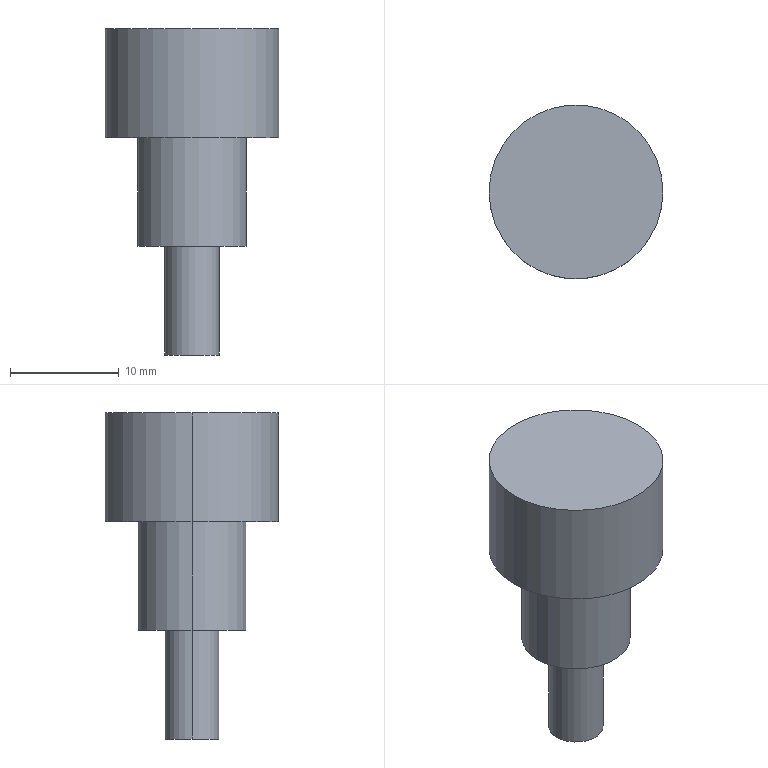Part | SolidWorks | features ICE 2, Extrusion 1 | 1 solid | 10 faces | box 16 x 16 x 30 mm | volume 2992 mm3 | cylinder 6 | plane 4 | commonest cylinder face diameters 5 x2 10 x2 16 x2
STEP:
#1=CARTESIAN_POINT('',(8.,0.,30.));
#2=VERTEX_POINT('',#1);
#3=CARTESIAN_POINT('',(-8.,0.,30.));
#4=VERTEX_POINT('',#3);
#5=CARTESIAN_POINT('',(0.,0.,30.));
#6=DIRECTION('',(0.,0.,1.));
#7=DIRECTION('',(1.,0.,0.));
#8=AXIS2_PLACEMENT_3D('',#5,#6,#7);
#9=CIRCLE('',#8,8.);
#10=EDGE_CURVE('',#2,#4,#9,.T.);
#11=ORIENTED_EDGE('',*,*,#10,.F.);
#12=CARTESIAN_POINT('',(8.,0.,20.));
#13=VERTEX_POINT('',#12);
#14=CARTESIAN_POINT('',(8.,0.,30.));
#15=DIRECTION('',(0.,0.,-1.));
#16=VECTOR('',#15,1000.);
#17=LINE('',#14,#16);
#18=EDGE_CURVE('',#2,#13,#17,.T.);
#19=ORIENTED_EDGE('',*,*,#18,.T.);
#20=CARTESIAN_POINT('',(-8.,0.,20.));
#21=VERTEX_POINT('',#20);
#22=CARTESIAN_POINT('',(0.,0.,20.));
#23=DIRECTION('',(0.,0.,1.));
#24=DIRECTION('',(1.,0.,0.));
#25=AXIS2_PLACEMENT_3D('',#22,#23,#24);
#26=CIRCLE('',#25,8.);
#27=EDGE_CURVE('',#13,#21,#26,.T.);
#28=ORIENTED_EDGE('',*,*,#27,.T.);
#29=CARTESIAN_POINT('',(-8.,0.,30.));
#30=DIRECTION('',(0.,0.,-1.));
#31=VECTOR('',#30,1000.);
#32=LINE('',#29,#31);
#33=EDGE_CURVE('',#4,#21,#32,.T.);
#34=ORIENTED_EDGE('',*,*,#33,.F.);
#35=EDGE_LOOP('',(#11,#19,#28,#34));
#36=FACE_OUTER_BOUND('',#35,.T.);
#37=CARTESIAN_POINT('',(0.,0.,30.));
#38=DIRECTION('',(0.,0.,-1.));
#39=DIRECTION('',(-1.,0.,0.));
#40=AXIS2_PLACEMENT_3D('',#37,#38,#39);
#41=CYLINDRICAL_SURFACE('',#40,8.);
#42=ADVANCED_FACE('',(#36),#41,.T.);
#43=CARTESIAN_POINT('',(5.,0.,20.));
#44=VERTEX_POINT('',#43);
#45=CARTESIAN_POINT('',(-5.,0.,20.));
#46=VERTEX_POINT('',#45);
#47=CARTESIAN_POINT('',(0.,0.,20.));
#48=DIRECTION('',(0.,0.,1.));
#49=DIRECTION('',(1.,0.,0.));
#50=AXIS2_PLACEMENT_3D('',#47,#48,#49);
#51=CIRCLE('',#50,5.);
#52=EDGE_CURVE('',#44,#46,#51,.T.);
#53=ORIENTED_EDGE('',*,*,#52,.F.);
#54=CARTESIAN_POINT('',(5.,0.,10.));
#55=VERTEX_POINT('',#54);
#56=CARTESIAN_POINT('',(5.,0.,20.));
#57=DIRECTION('',(0.,0.,-1.));
#58=VECTOR('',#57,1000.);
#59=LINE('',#56,#58);
#60=EDGE_CURVE('',#44,#55,#59,.T.);
#61=ORIENTED_EDGE('',*,*,#60,.T.);
#62=CARTESIAN_POINT('',(-5.,0.,10.));
#63=VERTEX_POINT('',#62);
#64=CARTESIAN_POINT('',(0.,0.,10.));
#65=DIRECTION('',(0.,0.,1.));
#66=DIRECTION('',(1.,0.,0.));
#67=AXIS2_PLACEMENT_3D('',#64,#65,#66);
#68=CIRCLE('',#67,5.);
#69=EDGE_CURVE('',#55,#63,#68,.T.);
#70=ORIENTED_EDGE('',*,*,#69,.T.);
#71=CARTESIAN_POINT('',(-5.,0.,20.));
#72=DIRECTION('',(0.,0.,-1.));
#73=VECTOR('',#72,1000.);
#74=LINE('',#71,#73);
#75=EDGE_CURVE('',#46,#63,#74,.T.);
#76=ORIENTED_EDGE('',*,*,#75,.F.);
#77=EDGE_LOOP('',(#53,#61,#70,#76));
#78=FACE_OUTER_BOUND('',#77,.T.);
#79=CARTESIAN_POINT('',(0.,0.,20.));
#80=DIRECTION('',(0.,0.,-1.));
#81=DIRECTION('',(-1.,0.,0.));
#82=AXIS2_PLACEMENT_3D('',#79,#80,#81);
#83=CYLINDRICAL_SURFACE('',#82,5.);
#84=ADVANCED_FACE('',(#78),#83,.T.);
#85=CARTESIAN_POINT('',(2.5,0.,10.));
#86=VERTEX_POINT('',#85);
#87=CARTESIAN_POINT('',(-2.5,0.,10.));
#88=VERTEX_POINT('',#87);
#89=CARTESIAN_POINT('',(0.,0.,10.));
#90=DIRECTION('',(0.,0.,1.));
#91=DIRECTION('',(1.,0.,0.));
#92=AXIS2_PLACEMENT_3D('',#89,#90,#91);
#93=CIRCLE('',#92,2.5);
#94=EDGE_CURVE('',#86,#88,#93,.T.);
#95=ORIENTED_EDGE('',*,*,#94,.F.);
#96=CARTESIAN_POINT('',(2.5,0.,0.));
#97=VERTEX_POINT('',#96);
#98=CARTESIAN_POINT('',(2.5,0.,10.));
#99=DIRECTION('',(0.,0.,-1.));
#100=VECTOR('',#99,1000.);
#101=LINE('',#98,#100);
#102=EDGE_CURVE('',#86,#97,#101,.T.);
#103=ORIENTED_EDGE('',*,*,#102,.T.);
#104=CARTESIAN_POINT('',(-2.5,0.,0.));
#105=VERTEX_POINT('',#104);
#106=CARTESIAN_POINT('',(0.,0.,0.));
#107=DIRECTION('',(0.,0.,1.));
#108=DIRECTION('',(1.,0.,0.));
#109=AXIS2_PLACEMENT_3D('',#106,#107,#108);
#110=CIRCLE('',#109,2.5);
#111=EDGE_CURVE('',#97,#105,#110,.T.);
#112=ORIENTED_EDGE('',*,*,#111,.T.);
#113=CARTESIAN_POINT('',(-2.5,0.,10.));
#114=DIRECTION('',(0.,0.,-1.));
#115=VECTOR('',#114,1000.);
#116=LINE('',#113,#115);
#117=EDGE_CURVE('',#88,#105,#116,.T.);
#118=ORIENTED_EDGE('',*,*,#117,.F.);
#119=EDGE_LOOP('',(#95,#103,#112,#118));
#120=FACE_OUTER_BOUND('',#119,.T.);
#121=CARTESIAN_POINT('',(0.,0.,10.));
#122=DIRECTION('',(0.,0.,-1.));
#123=DIRECTION('',(-1.,0.,0.));
#124=AXIS2_PLACEMENT_3D('',#121,#122,#123);
#125=CYLINDRICAL_SURFACE('',#124,2.5);
#126=ADVANCED_FACE('',(#120),#125,.T.);
#127=ORIENTED_EDGE('',*,*,#102,.F.);
#128=CARTESIAN_POINT('',(0.,0.,10.));
#129=DIRECTION('',(0.,0.,1.));
#130=DIRECTION('',(1.,0.,0.));
#131=AXIS2_PLACEMENT_3D('',#128,#129,#130);
#132=CIRCLE('',#131,2.5);
#133=EDGE_CURVE('',#88,#86,#132,.T.);
#134=ORIENTED_EDGE('',*,*,#133,.F.);
#135=ORIENTED_EDGE('',*,*,#117,.T.);
#136=CARTESIAN_POINT('',(0.,0.,0.));
#137=DIRECTION('',(0.,0.,1.));
#138=DIRECTION('',(1.,0.,0.));
#139=AXIS2_PLACEMENT_3D('',#136,#137,#138);
#140=CIRCLE('',#139,2.5);
#141=EDGE_CURVE('',#105,#97,#140,.T.);
#142=ORIENTED_EDGE('',*,*,#141,.T.);
#143=EDGE_LOOP('',(#127,#134,#135,#142));
#144=FACE_OUTER_BOUND('',#143,.T.);
#145=CARTESIAN_POINT('',(0.,0.,10.));
#146=DIRECTION('',(0.,0.,-1.));
#147=DIRECTION('',(-1.,0.,0.));
#148=AXIS2_PLACEMENT_3D('',#145,#146,#147);
#149=CYLINDRICAL_SURFACE('',#148,2.5);
#150=ADVANCED_FACE('',(#144),#149,.T.);
#151=ORIENTED_EDGE('',*,*,#141,.F.);
#152=ORIENTED_EDGE('',*,*,#111,.F.);
#153=EDGE_LOOP('',(#151,#152));
#154=FACE_OUTER_BOUND('',#153,.T.);
#155=CARTESIAN_POINT('',(0.,0.,0.));
#156=DIRECTION('',(0.,0.,1.));
#157=DIRECTION('',(1.,0.,0.));
#158=AXIS2_PLACEMENT_3D('',#155,#156,#157);
#159=PLANE('',#158);
#160=ADVANCED_FACE('',(#154),#159,.F.);
#161=ORIENTED_EDGE('',*,*,#60,.F.);
#162=CARTESIAN_POINT('',(0.,0.,20.));
#163=DIRECTION('',(0.,0.,1.));
#164=DIRECTION('',(1.,0.,0.));
#165=AXIS2_PLACEMENT_3D('',#162,#163,#164);
#166=CIRCLE('',#165,5.);
#167=EDGE_CURVE('',#46,#44,#166,.T.);
#168=ORIENTED_EDGE('',*,*,#167,.F.);
#169=ORIENTED_EDGE('',*,*,#75,.T.);
#170=CARTESIAN_POINT('',(0.,0.,10.));
#171=DIRECTION('',(0.,0.,1.));
#172=DIRECTION('',(1.,0.,0.));
#173=AXIS2_PLACEMENT_3D('',#170,#171,#172);
#174=CIRCLE('',#173,5.);
#175=EDGE_CURVE('',#63,#55,#174,.T.);
#176=ORIENTED_EDGE('',*,*,#175,.T.);
#177=EDGE_LOOP('',(#161,#168,#169,#176));
#178=FACE_OUTER_BOUND('',#177,.T.);
#179=CARTESIAN_POINT('',(0.,0.,20.));
#180=DIRECTION('',(0.,0.,-1.));
#181=DIRECTION('',(-1.,0.,0.));
#182=AXIS2_PLACEMENT_3D('',#179,#180,#181);
#183=CYLINDRICAL_SURFACE('',#182,5.);
#184=ADVANCED_FACE('',(#178),#183,.T.);
#185=ORIENTED_EDGE('',*,*,#133,.T.);
#186=ORIENTED_EDGE('',*,*,#94,.T.);
#187=EDGE_LOOP('',(#185,#186));
#188=FACE_BOUND('',#187,.T.);
#189=ORIENTED_EDGE('',*,*,#175,.F.);
#190=ORIENTED_EDGE('',*,*,#69,.F.);
#191=EDGE_LOOP('',(#189,#190));
#192=FACE_OUTER_BOUND('',#191,.T.);
#193=CARTESIAN_POINT('',(0.,0.,10.));
#194=DIRECTION('',(0.,0.,1.));
#195=DIRECTION('',(1.,0.,0.));
#196=AXIS2_PLACEMENT_3D('',#193,#194,#195);
#197=PLANE('',#196);
#198=ADVANCED_FACE('',(#188,#192),#197,.F.);
#199=ORIENTED_EDGE('',*,*,#18,.F.);
#200=CARTESIAN_POINT('',(0.,0.,30.));
#201=DIRECTION('',(0.,0.,1.));
#202=DIRECTION('',(1.,0.,0.));
#203=AXIS2_PLACEMENT_3D('',#200,#201,#202);
#204=CIRCLE('',#203,8.);
#205=EDGE_CURVE('',#4,#2,#204,.T.);
#206=ORIENTED_EDGE('',*,*,#205,.F.);
#207=ORIENTED_EDGE('',*,*,#33,.T.);
#208=CARTESIAN_POINT('',(0.,0.,20.));
#209=DIRECTION('',(0.,0.,1.));
#210=DIRECTION('',(1.,0.,0.));
#211=AXIS2_PLACEMENT_3D('',#208,#209,#210);
#212=CIRCLE('',#211,8.);
#213=EDGE_CURVE('',#21,#13,#212,.T.);
#214=ORIENTED_EDGE('',*,*,#213,.T.);
#215=EDGE_LOOP('',(#199,#206,#207,#214));
#216=FACE_OUTER_BOUND('',#215,.T.);
#217=CARTESIAN_POINT('',(0.,0.,30.));
#218=DIRECTION('',(0.,0.,-1.));
#219=DIRECTION('',(-1.,0.,0.));
#220=AXIS2_PLACEMENT_3D('',#217,#218,#219);
#221=CYLINDRICAL_SURFACE('',#220,8.);
#222=ADVANCED_FACE('',(#216),#221,.T.);
#223=ORIENTED_EDGE('',*,*,#205,.T.);
#224=ORIENTED_EDGE('',*,*,#10,.T.);
#225=EDGE_LOOP('',(#223,#224));
#226=FACE_OUTER_BOUND('',#225,.T.);
#227=CARTESIAN_POINT('',(0.,0.,30.));
#228=DIRECTION('',(0.,0.,1.));
#229=DIRECTION('',(1.,0.,0.));
#230=AXIS2_PLACEMENT_3D('',#227,#228,#229);
#231=PLANE('',#230);
#232=ADVANCED_FACE('',(#226),#231,.T.);
#233=ORIENTED_EDGE('',*,*,#167,.T.);
#234=ORIENTED_EDGE('',*,*,#52,.T.);
#235=EDGE_LOOP('',(#233,#234));
#236=FACE_BOUND('',#235,.T.);
#237=ORIENTED_EDGE('',*,*,#213,.F.);
#238=ORIENTED_EDGE('',*,*,#27,.F.);
#239=EDGE_LOOP('',(#237,#238));
#240=FACE_OUTER_BOUND('',#239,.T.);
#241=CARTESIAN_POINT('',(0.,0.,20.));
#242=DIRECTION('',(0.,0.,1.));
#243=DIRECTION('',(1.,0.,0.));
#244=AXIS2_PLACEMENT_3D('',#241,#242,#243);
#245=PLANE('',#244);
#246=ADVANCED_FACE('',(#236,#240),#245,.F.);
#247=CLOSED_SHELL('',(#42,#84,#126,#150,#160,#184,#198,#222,#232,#246));
#248=MANIFOLD_SOLID_BREP('',#247);
#249=CARTESIAN_POINT('',(0.,0.,0.));
#250=DIRECTION('',(0.,0.,1.));
#251=DIRECTION('',(1.,0.,0.));
#252=AXIS2_PLACEMENT_3D('',#249,#250,#251);
#253=(LENGTH_UNIT()NAMED_UNIT(*)SI_UNIT(.MILLI.,.METRE.));
#254=UNCERTAINTY_MEASURE_WITH_UNIT(LENGTH_MEASURE(0.00001),#253,'','');
#255=(NAMED_UNIT(*)PLANE_ANGLE_UNIT()SI_UNIT($,.RADIAN.));
#256=(NAMED_UNIT(*)SI_UNIT($,.STERADIAN.)SOLID_ANGLE_UNIT());
#257=(GEOMETRIC_REPRESENTATION_CONTEXT(3)GLOBAL_UNCERTAINTY_ASSIGNED_CONTEXT((#254))GLOBAL_UNIT_ASSIGNED_CONTEXT((#253,#255,#256))REPRESENTATION_CONTEXT('',''));
#258=ADVANCED_BREP_SHAPE_REPRESENTATION('',(#248,#252),#257);